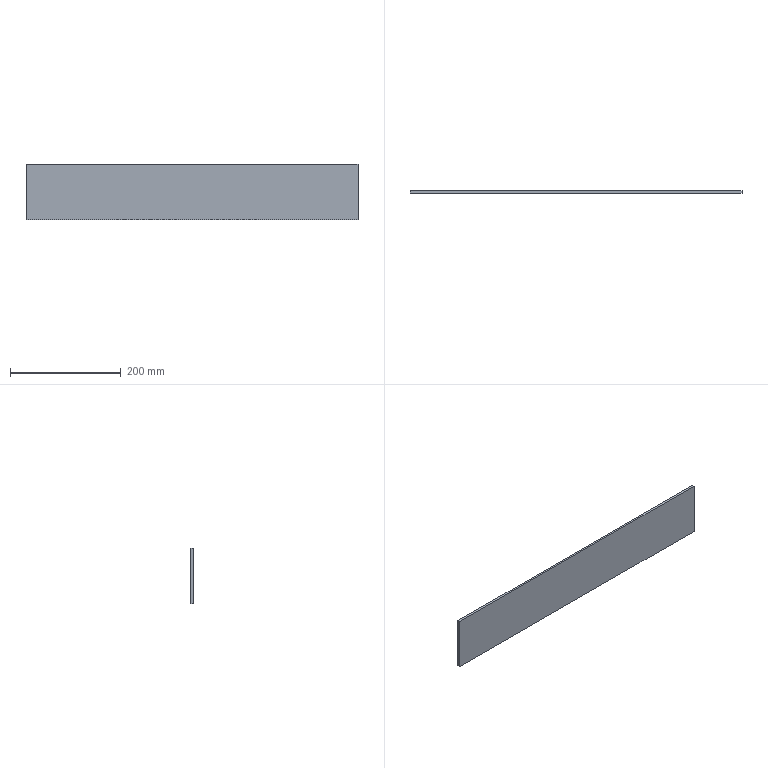Part | SolidWorks | features Extrusion 1 | 1 solid | 6 faces | box 600 x 4 x 100 mm | volume 240000 mm3 | plane 6
STEP:
#1=CARTESIAN_POINT('',(0.,0.,-100.));
#2=VERTEX_POINT('',#1);
#3=CARTESIAN_POINT('',(0.,0.,0.));
#4=VERTEX_POINT('',#3);
#5=CARTESIAN_POINT('',(0.,0.,0.));
#6=DIRECTION('',(0.,0.,1.));
#7=VECTOR('',#6,1000.);
#8=LINE('',#5,#7);
#9=EDGE_CURVE('',#2,#4,#8,.T.);
#10=ORIENTED_EDGE('',*,*,#9,.T.);
#11=CARTESIAN_POINT('',(0.,4.,0.));
#12=VERTEX_POINT('',#11);
#13=CARTESIAN_POINT('',(0.,4.,0.));
#14=DIRECTION('',(0.,-1.,0.));
#15=VECTOR('',#14,1000.);
#16=LINE('',#13,#15);
#17=EDGE_CURVE('',#12,#4,#16,.T.);
#18=ORIENTED_EDGE('',*,*,#17,.F.);
#19=CARTESIAN_POINT('',(0.,4.,-100.));
#20=VERTEX_POINT('',#19);
#21=CARTESIAN_POINT('',(0.,4.,0.));
#22=DIRECTION('',(0.,0.,1.));
#23=VECTOR('',#22,1000.);
#24=LINE('',#21,#23);
#25=EDGE_CURVE('',#20,#12,#24,.T.);
#26=ORIENTED_EDGE('',*,*,#25,.F.);
#27=CARTESIAN_POINT('',(0.,4.,-100.));
#28=DIRECTION('',(0.,-1.,0.));
#29=VECTOR('',#28,1000.);
#30=LINE('',#27,#29);
#31=EDGE_CURVE('',#20,#2,#30,.T.);
#32=ORIENTED_EDGE('',*,*,#31,.T.);
#33=EDGE_LOOP('',(#10,#18,#26,#32));
#34=FACE_OUTER_BOUND('',#33,.T.);
#35=CARTESIAN_POINT('',(0.,4.,0.));
#36=DIRECTION('',(1.,0.,0.));
#37=DIRECTION('',(0.,0.,-1.));
#38=AXIS2_PLACEMENT_3D('',#35,#36,#37);
#39=PLANE('',#38);
#40=ADVANCED_FACE('',(#34),#39,.F.);
#41=CARTESIAN_POINT('',(600.,0.,0.));
#42=VERTEX_POINT('',#41);
#43=CARTESIAN_POINT('',(0.,0.,0.));
#44=DIRECTION('',(1.,0.,0.));
#45=VECTOR('',#44,1000.);
#46=LINE('',#43,#45);
#47=EDGE_CURVE('',#4,#42,#46,.T.);
#48=ORIENTED_EDGE('',*,*,#47,.T.);
#49=CARTESIAN_POINT('',(600.,4.,0.));
#50=VERTEX_POINT('',#49);
#51=CARTESIAN_POINT('',(600.,4.,0.));
#52=DIRECTION('',(0.,-1.,0.));
#53=VECTOR('',#52,1000.);
#54=LINE('',#51,#53);
#55=EDGE_CURVE('',#50,#42,#54,.T.);
#56=ORIENTED_EDGE('',*,*,#55,.F.);
#57=CARTESIAN_POINT('',(0.,4.,0.));
#58=DIRECTION('',(1.,0.,0.));
#59=VECTOR('',#58,1000.);
#60=LINE('',#57,#59);
#61=EDGE_CURVE('',#12,#50,#60,.T.);
#62=ORIENTED_EDGE('',*,*,#61,.F.);
#63=ORIENTED_EDGE('',*,*,#17,.T.);
#64=EDGE_LOOP('',(#48,#56,#62,#63));
#65=FACE_OUTER_BOUND('',#64,.T.);
#66=CARTESIAN_POINT('',(0.,4.,0.));
#67=DIRECTION('',(0.,0.,-1.));
#68=DIRECTION('',(-1.,0.,0.));
#69=AXIS2_PLACEMENT_3D('',#66,#67,#68);
#70=PLANE('',#69);
#71=ADVANCED_FACE('',(#65),#70,.F.);
#72=CARTESIAN_POINT('',(600.,0.,-100.));
#73=VERTEX_POINT('',#72);
#74=CARTESIAN_POINT('',(600.,0.,0.));
#75=DIRECTION('',(0.,0.,-1.));
#76=VECTOR('',#75,1000.);
#77=LINE('',#74,#76);
#78=EDGE_CURVE('',#42,#73,#77,.T.);
#79=ORIENTED_EDGE('',*,*,#78,.T.);
#80=CARTESIAN_POINT('',(600.,4.,-100.));
#81=VERTEX_POINT('',#80);
#82=CARTESIAN_POINT('',(600.,4.,-100.));
#83=DIRECTION('',(0.,-1.,0.));
#84=VECTOR('',#83,1000.);
#85=LINE('',#82,#84);
#86=EDGE_CURVE('',#81,#73,#85,.T.);
#87=ORIENTED_EDGE('',*,*,#86,.F.);
#88=CARTESIAN_POINT('',(600.,4.,0.));
#89=DIRECTION('',(0.,0.,-1.));
#90=VECTOR('',#89,1000.);
#91=LINE('',#88,#90);
#92=EDGE_CURVE('',#50,#81,#91,.T.);
#93=ORIENTED_EDGE('',*,*,#92,.F.);
#94=ORIENTED_EDGE('',*,*,#55,.T.);
#95=EDGE_LOOP('',(#79,#87,#93,#94));
#96=FACE_OUTER_BOUND('',#95,.T.);
#97=CARTESIAN_POINT('',(600.,4.,0.));
#98=DIRECTION('',(-1.,0.,0.));
#99=DIRECTION('',(0.,0.,1.));
#100=AXIS2_PLACEMENT_3D('',#97,#98,#99);
#101=PLANE('',#100);
#102=ADVANCED_FACE('',(#96),#101,.F.);
#103=CARTESIAN_POINT('',(0.,0.,-100.));
#104=DIRECTION('',(-1.,0.,0.));
#105=VECTOR('',#104,1000.);
#106=LINE('',#103,#105);
#107=EDGE_CURVE('',#73,#2,#106,.T.);
#108=ORIENTED_EDGE('',*,*,#107,.T.);
#109=ORIENTED_EDGE('',*,*,#31,.F.);
#110=CARTESIAN_POINT('',(0.,4.,-100.));
#111=DIRECTION('',(-1.,0.,0.));
#112=VECTOR('',#111,1000.);
#113=LINE('',#110,#112);
#114=EDGE_CURVE('',#81,#20,#113,.T.);
#115=ORIENTED_EDGE('',*,*,#114,.F.);
#116=ORIENTED_EDGE('',*,*,#86,.T.);
#117=EDGE_LOOP('',(#108,#109,#115,#116));
#118=FACE_OUTER_BOUND('',#117,.T.);
#119=CARTESIAN_POINT('',(0.,4.,-100.));
#120=DIRECTION('',(0.,0.,1.));
#121=DIRECTION('',(1.,0.,0.));
#122=AXIS2_PLACEMENT_3D('',#119,#120,#121);
#123=PLANE('',#122);
#124=ADVANCED_FACE('',(#118),#123,.F.);
#125=ORIENTED_EDGE('',*,*,#25,.T.);
#126=ORIENTED_EDGE('',*,*,#61,.T.);
#127=ORIENTED_EDGE('',*,*,#92,.T.);
#128=ORIENTED_EDGE('',*,*,#114,.T.);
#129=EDGE_LOOP('',(#125,#126,#127,#128));
#130=FACE_OUTER_BOUND('',#129,.T.);
#131=CARTESIAN_POINT('',(0.,4.,0.));
#132=DIRECTION('',(0.,-1.,0.));
#133=DIRECTION('',(0.,0.,-1.));
#134=AXIS2_PLACEMENT_3D('',#131,#132,#133);
#135=PLANE('',#134);
#136=ADVANCED_FACE('',(#130),#135,.F.);
#137=ORIENTED_EDGE('',*,*,#9,.F.);
#138=ORIENTED_EDGE('',*,*,#107,.F.);
#139=ORIENTED_EDGE('',*,*,#78,.F.);
#140=ORIENTED_EDGE('',*,*,#47,.F.);
#141=EDGE_LOOP('',(#137,#138,#139,#140));
#142=FACE_OUTER_BOUND('',#141,.T.);
#143=CARTESIAN_POINT('',(0.,0.,0.));
#144=DIRECTION('',(0.,-1.,0.));
#145=DIRECTION('',(0.,0.,-1.));
#146=AXIS2_PLACEMENT_3D('',#143,#144,#145);
#147=PLANE('',#146);
#148=ADVANCED_FACE('',(#142),#147,.T.);
#149=CLOSED_SHELL('',(#40,#71,#102,#124,#136,#148));
#150=MANIFOLD_SOLID_BREP('',#149);
#151=CARTESIAN_POINT('',(0.,0.,0.));
#152=DIRECTION('',(0.,0.,1.));
#153=DIRECTION('',(1.,0.,0.));
#154=AXIS2_PLACEMENT_3D('',#151,#152,#153);
#155=(LENGTH_UNIT()NAMED_UNIT(*)SI_UNIT(.MILLI.,.METRE.));
#156=UNCERTAINTY_MEASURE_WITH_UNIT(LENGTH_MEASURE(0.00001),#155,'','');
#157=(NAMED_UNIT(*)PLANE_ANGLE_UNIT()SI_UNIT($,.RADIAN.));
#158=(NAMED_UNIT(*)SI_UNIT($,.STERADIAN.)SOLID_ANGLE_UNIT());
#159=(GEOMETRIC_REPRESENTATION_CONTEXT(3)GLOBAL_UNCERTAINTY_ASSIGNED_CONTEXT((#156))GLOBAL_UNIT_ASSIGNED_CONTEXT((#155,#157,#158))REPRESENTATION_CONTEXT('',''));
#160=ADVANCED_BREP_SHAPE_REPRESENTATION('',(#150,#154),#159);